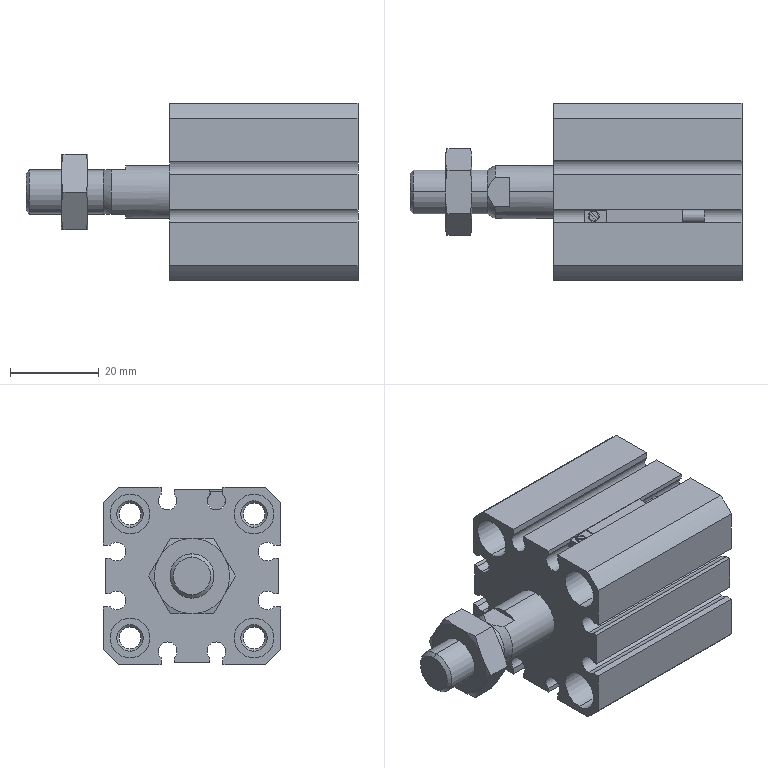Part | SolidWorks | features AEMSimFeature 1 | 4 solids | 216 faces | box 75 x 40 x 40 mm | volume 54113 mm3 | cylinder 88 | plane 68 | cone 60 | commonest cylinder face diameters 4.2 x18 4.917 x16 9 x16 5.4 x8 4.134 x4 12 x4